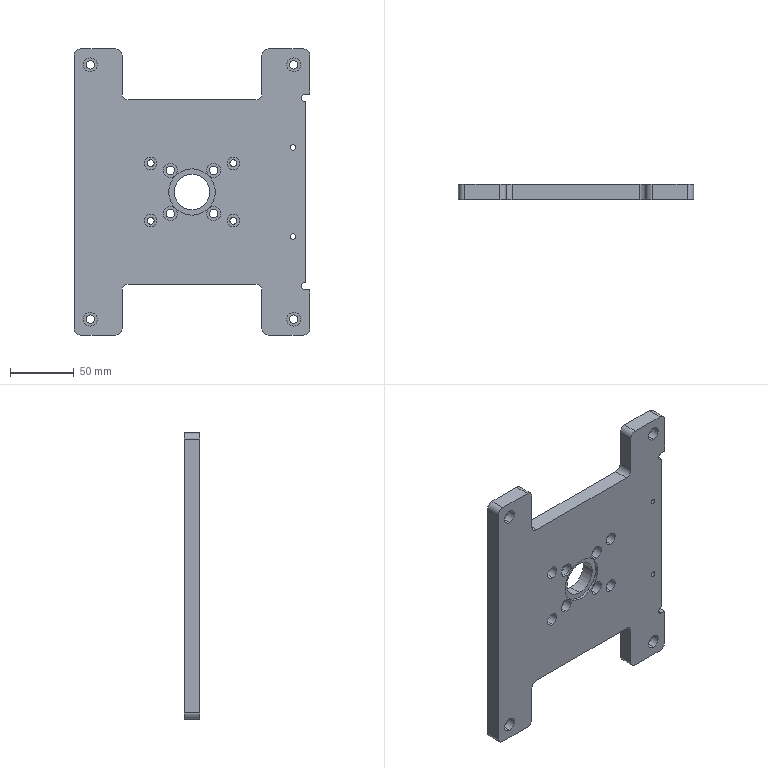Part | STEP file | 1 solid | 125 faces | box 185 x 12 x 225 mm | volume 366381 mm3 | cylinder 84 | plane 35 | cone 6 | commonest cylinder face diameters 10 x20 6.6 x16 11 x16 5.5 x8 20 x8 3.3 x6